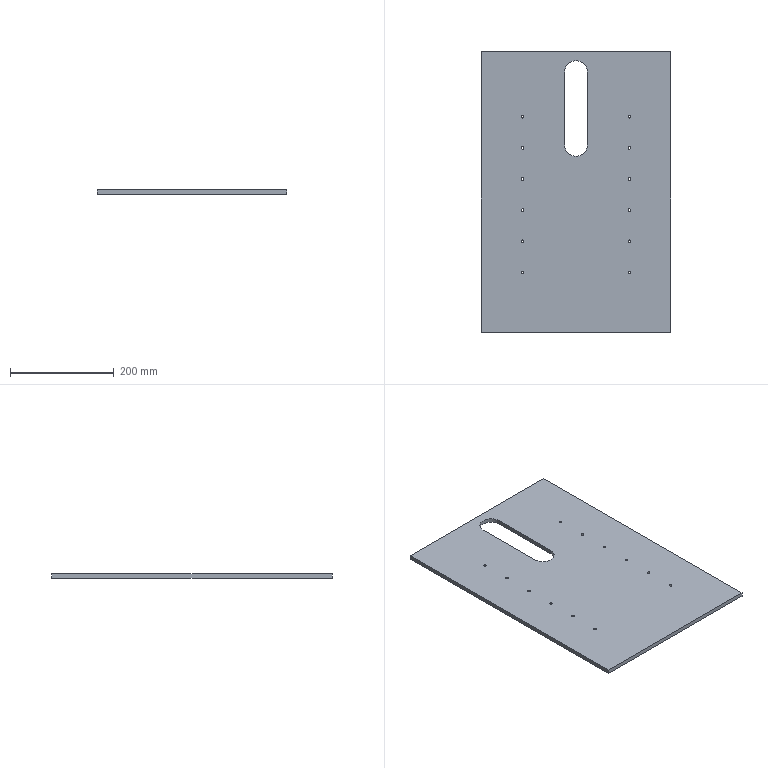Part | SolidWorks | features Extrusion 1, HoleWzd 1, LPattern 1 | 1 solid | 34 faces | box 365 x 540 x 8 mm | volume 1513471 mm3 | cylinder 26 | plane 8 | commonest cylinder face diameters 5 x24 44 x2
STEP:
#1=CARTESIAN_POINT('',(283.,-185.,0.));
#2=VERTEX_POINT('',#1);
#3=CARTESIAN_POINT('',(288.,-185.,0.));
#4=VERTEX_POINT('',#3);
#5=CARTESIAN_POINT('',(285.5,-185.,0.));
#6=DIRECTION('',(0.,0.,1.));
#7=DIRECTION('',(1.,0.,0.));
#8=AXIS2_PLACEMENT_3D('',#5,#6,#7);
#9=CIRCLE('',#8,2.5);
#10=EDGE_CURVE('',#2,#4,#9,.T.);
#11=ORIENTED_EDGE('',*,*,#10,.F.);
#12=CARTESIAN_POINT('',(283.,-185.,8.));
#13=VERTEX_POINT('',#12);
#14=CARTESIAN_POINT('',(283.,-185.,8.));
#15=DIRECTION('',(0.,0.,1.));
#16=VECTOR('',#15,1000.);
#17=LINE('',#14,#16);
#18=EDGE_CURVE('',#2,#13,#17,.T.);
#19=ORIENTED_EDGE('',*,*,#18,.T.);
#20=CARTESIAN_POINT('',(288.,-185.,8.));
#21=VERTEX_POINT('',#20);
#22=CARTESIAN_POINT('',(285.5,-185.,8.));
#23=DIRECTION('',(0.,0.,1.));
#24=DIRECTION('',(1.,0.,0.));
#25=AXIS2_PLACEMENT_3D('',#22,#23,#24);
#26=CIRCLE('',#25,2.5);
#27=EDGE_CURVE('',#13,#21,#26,.T.);
#28=ORIENTED_EDGE('',*,*,#27,.T.);
#29=CARTESIAN_POINT('',(288.,-185.,8.));
#30=DIRECTION('',(0.,0.,1.));
#31=VECTOR('',#30,1000.);
#32=LINE('',#29,#31);
#33=EDGE_CURVE('',#4,#21,#32,.T.);
#34=ORIENTED_EDGE('',*,*,#33,.F.);
#35=EDGE_LOOP('',(#11,#19,#28,#34));
#36=FACE_OUTER_BOUND('',#35,.T.);
#37=CARTESIAN_POINT('',(285.5,-185.,8.));
#38=DIRECTION('',(0.,0.,1.));
#39=DIRECTION('',(1.,0.,0.));
#40=AXIS2_PLACEMENT_3D('',#37,#38,#39);
#41=CYLINDRICAL_SURFACE('',#40,2.5);
#42=ADVANCED_FACE('',(#36),#41,.F.);
#43=CARTESIAN_POINT('',(77.,-185.,0.));
#44=VERTEX_POINT('',#43);
#45=CARTESIAN_POINT('',(82.,-185.,0.));
#46=VERTEX_POINT('',#45);
#47=CARTESIAN_POINT('',(79.5,-185.,0.));
#48=DIRECTION('',(0.,0.,1.));
#49=DIRECTION('',(1.,0.,0.));
#50=AXIS2_PLACEMENT_3D('',#47,#48,#49);
#51=CIRCLE('',#50,2.5);
#52=EDGE_CURVE('',#44,#46,#51,.T.);
#53=ORIENTED_EDGE('',*,*,#52,.F.);
#54=CARTESIAN_POINT('',(77.,-185.,8.));
#55=VERTEX_POINT('',#54);
#56=CARTESIAN_POINT('',(77.,-185.,8.));
#57=DIRECTION('',(0.,0.,1.));
#58=VECTOR('',#57,1000.);
#59=LINE('',#56,#58);
#60=EDGE_CURVE('',#44,#55,#59,.T.);
#61=ORIENTED_EDGE('',*,*,#60,.T.);
#62=CARTESIAN_POINT('',(82.,-185.,8.));
#63=VERTEX_POINT('',#62);
#64=CARTESIAN_POINT('',(79.5,-185.,8.));
#65=DIRECTION('',(0.,0.,1.));
#66=DIRECTION('',(1.,0.,0.));
#67=AXIS2_PLACEMENT_3D('',#64,#65,#66);
#68=CIRCLE('',#67,2.5);
#69=EDGE_CURVE('',#55,#63,#68,.T.);
#70=ORIENTED_EDGE('',*,*,#69,.T.);
#71=CARTESIAN_POINT('',(82.,-185.,8.));
#72=DIRECTION('',(0.,0.,1.));
#73=VECTOR('',#72,1000.);
#74=LINE('',#71,#73);
#75=EDGE_CURVE('',#46,#63,#74,.T.);
#76=ORIENTED_EDGE('',*,*,#75,.F.);
#77=EDGE_LOOP('',(#53,#61,#70,#76));
#78=FACE_OUTER_BOUND('',#77,.T.);
#79=CARTESIAN_POINT('',(79.5,-185.,8.));
#80=DIRECTION('',(0.,0.,1.));
#81=DIRECTION('',(1.,0.,0.));
#82=AXIS2_PLACEMENT_3D('',#79,#80,#81);
#83=CYLINDRICAL_SURFACE('',#82,2.5);
#84=ADVANCED_FACE('',(#78),#83,.F.);
#85=CARTESIAN_POINT('',(77.,-125.,0.));
#86=VERTEX_POINT('',#85);
#87=CARTESIAN_POINT('',(82.,-125.,0.));
#88=VERTEX_POINT('',#87);
#89=CARTESIAN_POINT('',(79.5,-125.,0.));
#90=DIRECTION('',(0.,0.,1.));
#91=DIRECTION('',(1.,0.,0.));
#92=AXIS2_PLACEMENT_3D('',#89,#90,#91);
#93=CIRCLE('',#92,2.5);
#94=EDGE_CURVE('',#86,#88,#93,.T.);
#95=ORIENTED_EDGE('',*,*,#94,.F.);
#96=CARTESIAN_POINT('',(77.,-125.,8.));
#97=VERTEX_POINT('',#96);
#98=CARTESIAN_POINT('',(77.,-125.,8.));
#99=DIRECTION('',(0.,0.,1.));
#100=VECTOR('',#99,1000.);
#101=LINE('',#98,#100);
#102=EDGE_CURVE('',#86,#97,#101,.T.);
#103=ORIENTED_EDGE('',*,*,#102,.T.);
#104=CARTESIAN_POINT('',(82.,-125.,8.));
#105=VERTEX_POINT('',#104);
#106=CARTESIAN_POINT('',(79.5,-125.,8.));
#107=DIRECTION('',(0.,0.,1.));
#108=DIRECTION('',(1.,0.,0.));
#109=AXIS2_PLACEMENT_3D('',#106,#107,#108);
#110=CIRCLE('',#109,2.5);
#111=EDGE_CURVE('',#97,#105,#110,.T.);
#112=ORIENTED_EDGE('',*,*,#111,.T.);
#113=CARTESIAN_POINT('',(82.,-125.,8.));
#114=DIRECTION('',(0.,0.,1.));
#115=VECTOR('',#114,1000.);
#116=LINE('',#113,#115);
#117=EDGE_CURVE('',#88,#105,#116,.T.);
#118=ORIENTED_EDGE('',*,*,#117,.F.);
#119=EDGE_LOOP('',(#95,#103,#112,#118));
#120=FACE_OUTER_BOUND('',#119,.T.);
#121=CARTESIAN_POINT('',(79.5,-125.,8.));
#122=DIRECTION('',(0.,0.,1.));
#123=DIRECTION('',(1.,0.,0.));
#124=AXIS2_PLACEMENT_3D('',#121,#122,#123);
#125=CYLINDRICAL_SURFACE('',#124,2.5);
#126=ADVANCED_FACE('',(#120),#125,.F.);
#127=CARTESIAN_POINT('',(283.,-125.,0.));
#128=VERTEX_POINT('',#127);
#129=CARTESIAN_POINT('',(288.,-125.,0.));
#130=VERTEX_POINT('',#129);
#131=CARTESIAN_POINT('',(285.5,-125.,0.));
#132=DIRECTION('',(0.,0.,1.));
#133=DIRECTION('',(1.,0.,0.));
#134=AXIS2_PLACEMENT_3D('',#131,#132,#133);
#135=CIRCLE('',#134,2.5);
#136=EDGE_CURVE('',#128,#130,#135,.T.);
#137=ORIENTED_EDGE('',*,*,#136,.F.);
#138=CARTESIAN_POINT('',(283.,-125.,8.));
#139=VERTEX_POINT('',#138);
#140=CARTESIAN_POINT('',(283.,-125.,8.));
#141=DIRECTION('',(0.,0.,1.));
#142=VECTOR('',#141,1000.);
#143=LINE('',#140,#142);
#144=EDGE_CURVE('',#128,#139,#143,.T.);
#145=ORIENTED_EDGE('',*,*,#144,.T.);
#146=CARTESIAN_POINT('',(288.,-125.,8.));
#147=VERTEX_POINT('',#146);
#148=CARTESIAN_POINT('',(285.5,-125.,8.));
#149=DIRECTION('',(0.,0.,1.));
#150=DIRECTION('',(1.,0.,0.));
#151=AXIS2_PLACEMENT_3D('',#148,#149,#150);
#152=CIRCLE('',#151,2.5);
#153=EDGE_CURVE('',#139,#147,#152,.T.);
#154=ORIENTED_EDGE('',*,*,#153,.T.);
#155=CARTESIAN_POINT('',(288.,-125.,8.));
#156=DIRECTION('',(0.,0.,1.));
#157=VECTOR('',#156,1000.);
#158=LINE('',#155,#157);
#159=EDGE_CURVE('',#130,#147,#158,.T.);
#160=ORIENTED_EDGE('',*,*,#159,.F.);
#161=EDGE_LOOP('',(#137,#145,#154,#160));
#162=FACE_OUTER_BOUND('',#161,.T.);
#163=CARTESIAN_POINT('',(285.5,-125.,8.));
#164=DIRECTION('',(0.,0.,1.));
#165=DIRECTION('',(1.,0.,0.));
#166=AXIS2_PLACEMENT_3D('',#163,#164,#165);
#167=CYLINDRICAL_SURFACE('',#166,2.5);
#168=ADVANCED_FACE('',(#162),#167,.F.);
#169=CARTESIAN_POINT('',(77.,-245.,0.));
#170=VERTEX_POINT('',#169);
#171=CARTESIAN_POINT('',(82.,-245.,0.));
#172=VERTEX_POINT('',#171);
#173=CARTESIAN_POINT('',(79.5,-245.,0.));
#174=DIRECTION('',(0.,0.,1.));
#175=DIRECTION('',(1.,0.,0.));
#176=AXIS2_PLACEMENT_3D('',#173,#174,#175);
#177=CIRCLE('',#176,2.5);
#178=EDGE_CURVE('',#170,#172,#177,.T.);
#179=ORIENTED_EDGE('',*,*,#178,.F.);
#180=CARTESIAN_POINT('',(77.,-245.,8.));
#181=VERTEX_POINT('',#180);
#182=CARTESIAN_POINT('',(77.,-245.,8.));
#183=DIRECTION('',(0.,0.,1.));
#184=VECTOR('',#183,1000.);
#185=LINE('',#182,#184);
#186=EDGE_CURVE('',#170,#181,#185,.T.);
#187=ORIENTED_EDGE('',*,*,#186,.T.);
#188=CARTESIAN_POINT('',(82.,-245.,8.));
#189=VERTEX_POINT('',#188);
#190=CARTESIAN_POINT('',(79.5,-245.,8.));
#191=DIRECTION('',(0.,0.,1.));
#192=DIRECTION('',(1.,0.,0.));
#193=AXIS2_PLACEMENT_3D('',#190,#191,#192);
#194=CIRCLE('',#193,2.5);
#195=EDGE_CURVE('',#181,#189,#194,.T.);
#196=ORIENTED_EDGE('',*,*,#195,.T.);
#197=CARTESIAN_POINT('',(82.,-245.,8.));
#198=DIRECTION('',(0.,0.,1.));
#199=VECTOR('',#198,1000.);
#200=LINE('',#197,#199);
#201=EDGE_CURVE('',#172,#189,#200,.T.);
#202=ORIENTED_EDGE('',*,*,#201,.F.);
#203=EDGE_LOOP('',(#179,#187,#196,#202));
#204=FACE_OUTER_BOUND('',#203,.T.);
#205=CARTESIAN_POINT('',(79.5,-245.,8.));
#206=DIRECTION('',(0.,0.,1.));
#207=DIRECTION('',(1.,0.,0.));
#208=AXIS2_PLACEMENT_3D('',#205,#206,#207);
#209=CYLINDRICAL_SURFACE('',#208,2.5);
#210=ADVANCED_FACE('',(#204),#209,.F.);
#211=CARTESIAN_POINT('',(77.,-305.,0.));
#212=VERTEX_POINT('',#211);
#213=CARTESIAN_POINT('',(82.,-305.,0.));
#214=VERTEX_POINT('',#213);
#215=CARTESIAN_POINT('',(79.5,-305.,0.));
#216=DIRECTION('',(0.,0.,1.));
#217=DIRECTION('',(1.,0.,0.));
#218=AXIS2_PLACEMENT_3D('',#215,#216,#217);
#219=CIRCLE('',#218,2.5);
#220=EDGE_CURVE('',#212,#214,#219,.T.);
#221=ORIENTED_EDGE('',*,*,#220,.F.);
#222=CARTESIAN_POINT('',(77.,-305.,8.));
#223=VERTEX_POINT('',#222);
#224=CARTESIAN_POINT('',(77.,-305.,8.));
#225=DIRECTION('',(0.,0.,1.));
#226=VECTOR('',#225,1000.);
#227=LINE('',#224,#226);
#228=EDGE_CURVE('',#212,#223,#227,.T.);
#229=ORIENTED_EDGE('',*,*,#228,.T.);
#230=CARTESIAN_POINT('',(82.,-305.,8.));
#231=VERTEX_POINT('',#230);
#232=CARTESIAN_POINT('',(79.5,-305.,8.));
#233=DIRECTION('',(0.,0.,1.));
#234=DIRECTION('',(1.,0.,0.));
#235=AXIS2_PLACEMENT_3D('',#232,#233,#234);
#236=CIRCLE('',#235,2.5);
#237=EDGE_CURVE('',#223,#231,#236,.T.);
#238=ORIENTED_EDGE('',*,*,#237,.T.);
#239=CARTESIAN_POINT('',(82.,-305.,8.));
#240=DIRECTION('',(0.,0.,1.));
#241=VECTOR('',#240,1000.);
#242=LINE('',#239,#241);
#243=EDGE_CURVE('',#214,#231,#242,.T.);
#244=ORIENTED_EDGE('',*,*,#243,.F.);
#245=EDGE_LOOP('',(#221,#229,#238,#244));
#246=FACE_OUTER_BOUND('',#245,.T.);
#247=CARTESIAN_POINT('',(79.5,-305.,8.));
#248=DIRECTION('',(0.,0.,1.));
#249=DIRECTION('',(1.,0.,0.));
#250=AXIS2_PLACEMENT_3D('',#247,#248,#249);
#251=CYLINDRICAL_SURFACE('',#250,2.5);
#252=ADVANCED_FACE('',(#246),#251,.F.);
#253=CARTESIAN_POINT('',(77.,-365.,0.));
#254=VERTEX_POINT('',#253);
#255=CARTESIAN_POINT('',(82.,-365.,0.));
#256=VERTEX_POINT('',#255);
#257=CARTESIAN_POINT('',(79.5,-365.,0.));
#258=DIRECTION('',(0.,0.,1.));
#259=DIRECTION('',(1.,0.,0.));
#260=AXIS2_PLACEMENT_3D('',#257,#258,#259);
#261=CIRCLE('',#260,2.5);
#262=EDGE_CURVE('',#254,#256,#261,.T.);
#263=ORIENTED_EDGE('',*,*,#262,.F.);
#264=CARTESIAN_POINT('',(77.,-365.,8.));
#265=VERTEX_POINT('',#264);
#266=CARTESIAN_POINT('',(77.,-365.,8.));
#267=DIRECTION('',(0.,0.,1.));
#268=VECTOR('',#267,1000.);
#269=LINE('',#266,#268);
#270=EDGE_CURVE('',#254,#265,#269,.T.);
#271=ORIENTED_EDGE('',*,*,#270,.T.);
#272=CARTESIAN_POINT('',(82.,-365.,8.));
#273=VERTEX_POINT('',#272);
#274=CARTESIAN_POINT('',(79.5,-365.,8.));
#275=DIRECTION('',(0.,0.,1.));
#276=DIRECTION('',(1.,0.,0.));
#277=AXIS2_PLACEMENT_3D('',#274,#275,#276);
#278=CIRCLE('',#277,2.5);
#279=EDGE_CURVE('',#265,#273,#278,.T.);
#280=ORIENTED_EDGE('',*,*,#279,.T.);
#281=CARTESIAN_POINT('',(82.,-365.,8.));
#282=DIRECTION('',(0.,0.,1.));
#283=VECTOR('',#282,1000.);
#284=LINE('',#281,#283);
#285=EDGE_CURVE('',#256,#273,#284,.T.);
#286=ORIENTED_EDGE('',*,*,#285,.F.);
#287=EDGE_LOOP('',(#263,#271,#280,#286));
#288=FACE_OUTER_BOUND('',#287,.T.);
#289=CARTESIAN_POINT('',(79.5,-365.,8.));
#290=DIRECTION('',(0.,0.,1.));
#291=DIRECTION('',(1.,0.,0.));
#292=AXIS2_PLACEMENT_3D('',#289,#290,#291);
#293=CYLINDRICAL_SURFACE('',#292,2.5);
#294=ADVANCED_FACE('',(#288),#293,.F.);
#295=CARTESIAN_POINT('',(77.,-425.,0.));
#296=VERTEX_POINT('',#295);
#297=CARTESIAN_POINT('',(82.,-425.,0.));
#298=VERTEX_POINT('',#297);
#299=CARTESIAN_POINT('',(79.5,-425.,0.));
#300=DIRECTION('',(0.,0.,1.));
#301=DIRECTION('',(1.,0.,0.));
#302=AXIS2_PLACEMENT_3D('',#299,#300,#301);
#303=CIRCLE('',#302,2.5);
#304=EDGE_CURVE('',#296,#298,#303,.T.);
#305=ORIENTED_EDGE('',*,*,#304,.F.);
#306=CARTESIAN_POINT('',(77.,-425.,8.));
#307=VERTEX_POINT('',#306);
#308=CARTESIAN_POINT('',(77.,-425.,8.));
#309=DIRECTION('',(0.,0.,1.));
#310=VECTOR('',#309,1000.);
#311=LINE('',#308,#310);
#312=EDGE_CURVE('',#296,#307,#311,.T.);
#313=ORIENTED_EDGE('',*,*,#312,.T.);
#314=CARTESIAN_POINT('',(82.,-425.,8.));
#315=VERTEX_POINT('',#314);
#316=CARTESIAN_POINT('',(79.5,-425.,8.));
#317=DIRECTION('',(0.,0.,1.));
#318=DIRECTION('',(1.,0.,0.));
#319=AXIS2_PLACEMENT_3D('',#316,#317,#318);
#320=CIRCLE('',#319,2.5);
#321=EDGE_CURVE('',#307,#315,#320,.T.);
#322=ORIENTED_EDGE('',*,*,#321,.T.);
#323=CARTESIAN_POINT('',(82.,-425.,8.));
#324=DIRECTION('',(0.,0.,1.));
#325=VECTOR('',#324,1000.);
#326=LINE('',#323,#325);
#327=EDGE_CURVE('',#298,#315,#326,.T.);
#328=ORIENTED_EDGE('',*,*,#327,.F.);
#329=EDGE_LOOP('',(#305,#313,#322,#328));
#330=FACE_OUTER_BOUND('',#329,.T.);
#331=CARTESIAN_POINT('',(79.5,-425.,8.));
#332=DIRECTION('',(0.,0.,1.));
#333=DIRECTION('',(1.,0.,0.));
#334=AXIS2_PLACEMENT_3D('',#331,#332,#333);
#335=CYLINDRICAL_SURFACE('',#334,2.5);
#336=ADVANCED_FACE('',(#330),#335,.F.);
#337=CARTESIAN_POINT('',(283.,-245.,0.));
#338=VERTEX_POINT('',#337);
#339=CARTESIAN_POINT('',(288.,-245.,0.));
#340=VERTEX_POINT('',#339);
#341=CARTESIAN_POINT('',(285.5,-245.,0.));
#342=DIRECTION('',(0.,0.,1.));
#343=DIRECTION('',(1.,0.,0.));
#344=AXIS2_PLACEMENT_3D('',#341,#342,#343);
#345=CIRCLE('',#344,2.5);
#346=EDGE_CURVE('',#338,#340,#345,.T.);
#347=ORIENTED_EDGE('',*,*,#346,.F.);
#348=CARTESIAN_POINT('',(283.,-245.,8.));
#349=VERTEX_POINT('',#348);
#350=CARTESIAN_POINT('',(283.,-245.,8.));
#351=DIRECTION('',(0.,0.,1.));
#352=VECTOR('',#351,1000.);
#353=LINE('',#350,#352);
#354=EDGE_CURVE('',#338,#349,#353,.T.);
#355=ORIENTED_EDGE('',*,*,#354,.T.);
#356=CARTESIAN_POINT('',(288.,-245.,8.));
#357=VERTEX_POINT('',#356);
#358=CARTESIAN_POINT('',(285.5,-245.,8.));
#359=DIRECTION('',(0.,0.,1.));
#360=DIRECTION('',(1.,0.,0.));
#361=AXIS2_PLACEMENT_3D('',#358,#359,#360);
#362=CIRCLE('',#361,2.5);
#363=EDGE_CURVE('',#349,#357,#362,.T.);
#364=ORIENTED_EDGE('',*,*,#363,.T.);
#365=CARTESIAN_POINT('',(288.,-245.,8.));
#366=DIRECTION('',(0.,0.,1.));
#367=VECTOR('',#366,1000.);
#368=LINE('',#365,#367);
#369=EDGE_CURVE('',#340,#357,#368,.T.);
#370=ORIENTED_EDGE('',*,*,#369,.F.);
#371=EDGE_LOOP('',(#347,#355,#364,#370));
#372=FACE_OUTER_BOUND('',#371,.T.);
#373=CARTESIAN_POINT('',(285.5,-245.,8.));
#374=DIRECTION('',(0.,0.,1.));
#375=DIRECTION('',(1.,0.,0.));
#376=AXIS2_PLACEMENT_3D('',#373,#374,#375);
#377=CYLINDRICAL_SURFACE('',#376,2.5);
#378=ADVANCED_FACE('',(#372),#377,.F.);
#379=CARTESIAN_POINT('',(283.,-305.,0.));
#380=VERTEX_POINT('',#379);
#381=CARTESIAN_POINT('',(288.,-305.,0.));
#382=VERTEX_POINT('',#381);
#383=CARTESIAN_POINT('',(285.5,-305.,0.));
#384=DIRECTION('',(0.,0.,1.));
#385=DIRECTION('',(1.,0.,0.));
#386=AXIS2_PLACEMENT_3D('',#383,#384,#385);
#387=CIRCLE('',#386,2.5);
#388=EDGE_CURVE('',#380,#382,#387,.T.);
#389=ORIENTED_EDGE('',*,*,#388,.F.);
#390=CARTESIAN_POINT('',(283.,-305.,8.));
#391=VERTEX_POINT('',#390);
#392=CARTESIAN_POINT('',(283.,-305.,8.));
#393=DIRECTION('',(0.,0.,1.));
#394=VECTOR('',#393,1000.);
#395=LINE('',#392,#394);
#396=EDGE_CURVE('',#380,#391,#395,.T.);
#397=ORIENTED_EDGE('',*,*,#396,.T.);
#398=CARTESIAN_POINT('',(288.,-305.,8.));
#399=VERTEX_POINT('',#398);
#400=CARTESIAN_POINT('',(285.5,-305.,8.));
#401=DIRECTION('',(0.,0.,1.));
#402=DIRECTION('',(1.,0.,0.));
#403=AXIS2_PLACEMENT_3D('',#400,#401,#402);
#404=CIRCLE('',#403,2.5);
#405=EDGE_CURVE('',#391,#399,#404,.T.);
#406=ORIENTED_EDGE('',*,*,#405,.T.);
#407=CARTESIAN_POINT('',(288.,-305.,8.));
#408=DIRECTION('',(0.,0.,1.));
#409=VECTOR('',#408,1000.);
#410=LINE('',#407,#409);
#411=EDGE_CURVE('',#382,#399,#410,.T.);
#412=ORIENTED_EDGE('',*,*,#411,.F.);
#413=EDGE_LOOP('',(#389,#397,#406,#412));
#414=FACE_OUTER_BOUND('',#413,.T.);
#415=CARTESIAN_POINT('',(285.5,-305.,8.));
#416=DIRECTION('',(0.,0.,1.));
#417=DIRECTION('',(1.,0.,0.));
#418=AXIS2_PLACEMENT_3D('',#415,#416,#417);
#419=CYLINDRICAL_SURFACE('',#418,2.5);
#420=ADVANCED_FACE('',(#414),#419,.F.);
#421=CARTESIAN_POINT('',(283.,-365.,0.));
#422=VERTEX_POINT('',#421);
#423=CARTESIAN_POINT('',(288.,-365.,0.));
#424=VERTEX_POINT('',#423);
#425=CARTESIAN_POINT('',(285.5,-365.,0.));
#426=DIRECTION('',(0.,0.,1.));
#427=DIRECTION('',(1.,0.,0.));
#428=AXIS2_PLACEMENT_3D('',#425,#426,#427);
#429=CIRCLE('',#428,2.5);
#430=EDGE_CURVE('',#422,#424,#429,.T.);
#431=ORIENTED_EDGE('',*,*,#430,.F.);
#432=CARTESIAN_POINT('',(283.,-365.,8.));
#433=VERTEX_POINT('',#432);
#434=CARTESIAN_POINT('',(283.,-365.,8.));
#435=DIRECTION('',(0.,0.,1.));
#436=VECTOR('',#435,1000.);
#437=LINE('',#434,#436);
#438=EDGE_CURVE('',#422,#433,#437,.T.);
#439=ORIENTED_EDGE('',*,*,#438,.T.);
#440=CARTESIAN_POINT('',(288.,-365.,8.));
#441=VERTEX_POINT('',#440);
#442=CARTESIAN_POINT('',(285.5,-365.,8.));
#443=DIRECTION('',(0.,0.,1.));
#444=DIRECTION('',(1.,0.,0.));
#445=AXIS2_PLACEMENT_3D('',#442,#443,#444);
#446=CIRCLE('',#445,2.5);
#447=EDGE_CURVE('',#433,#441,#446,.T.);
#448=ORIENTED_EDGE('',*,*,#447,.T.);
#449=CARTESIAN_POINT('',(288.,-365.,8.));
#450=DIRECTION('',(0.,0.,1.));
#451=VECTOR('',#450,1000.);
#452=LINE('',#449,#451);
#453=EDGE_CURVE('',#424,#441,#452,.T.);
#454=ORIENTED_EDGE('',*,*,#453,.F.);
#455=EDGE_LOOP('',(#431,#439,#448,#454));
#456=FACE_OUTER_BOUND('',#455,.T.);
#457=CARTESIAN_POINT('',(285.5,-365.,8.));
#458=DIRECTION('',(0.,0.,1.));
#459=DIRECTION('',(1.,0.,0.));
#460=AXIS2_PLACEMENT_3D('',#457,#458,#459);
#461=CYLINDRICAL_SURFACE('',#460,2.5);
#462=ADVANCED_FACE('',(#456),#461,.F.);
#463=CARTESIAN_POINT('',(283.,-425.,0.));
#464=VERTEX_POINT('',#463);
#465=CARTESIAN_POINT('',(288.,-425.,0.));
#466=VERTEX_POINT('',#465);
#467=CARTESIAN_POINT('',(285.5,-425.,0.));
#468=DIRECTION('',(0.,0.,1.));
#469=DIRECTION('',(1.,0.,0.));
#470=AXIS2_PLACEMENT_3D('',#467,#468,#469);
#471=CIRCLE('',#470,2.5);
#472=EDGE_CURVE('',#464,#466,#471,.T.);
#473=ORIENTED_EDGE('',*,*,#472,.F.);
#474=CARTESIAN_POINT('',(283.,-425.,8.));
#475=VERTEX_POINT('',#474);
#476=CARTESIAN_POINT('',(283.,-425.,8.));
#477=DIRECTION('',(0.,0.,1.));
#478=VECTOR('',#477,1000.);
#479=LINE('',#476,#478);
#480=EDGE_CURVE('',#464,#475,#479,.T.);
#481=ORIENTED_EDGE('',*,*,#480,.T.);
#482=CARTESIAN_POINT('',(288.,-425.,8.));
#483=VERTEX_POINT('',#482);
#484=CARTESIAN_POINT('',(285.5,-425.,8.));
#485=DIRECTION('',(0.,0.,1.));
#486=DIRECTION('',(1.,0.,0.));
#487=AXIS2_PLACEMENT_3D('',#484,#485,#486);
#488=CIRCLE('',#487,2.5);
#489=EDGE_CURVE('',#475,#483,#488,.T.);
#490=ORIENTED_EDGE('',*,*,#489,.T.);
#491=CARTESIAN_POINT('',(288.,-425.,8.));
#492=DIRECTION('',(0.,0.,1.));
#493=VECTOR('',#492,1000.);
#494=LINE('',#491,#493);
#495=EDGE_CURVE('',#466,#483,#494,.T.);
#496=ORIENTED_EDGE('',*,*,#495,.F.);
#497=EDGE_LOOP('',(#473,#481,#490,#496));
#498=FACE_OUTER_BOUND('',#497,.T.);
#499=CARTESIAN_POINT('',(285.5,-425.,8.));
#500=DIRECTION('',(0.,0.,1.));
#501=DIRECTION('',(1.,0.,0.));
#502=AXIS2_PLACEMENT_3D('',#499,#500,#501);
#503=CYLINDRICAL_SURFACE('',#502,2.5);
#504=ADVANCED_FACE('',(#498),#503,.F.);
#505=ORIENTED_EDGE('',*,*,#480,.F.);
#506=CARTESIAN_POINT('',(285.5,-425.,0.));
#507=DIRECTION('',(0.,0.,1.));
#508=DIRECTION('',(1.,0.,0.));
#509=AXIS2_PLACEMENT_3D('',#506,#507,#508);
#510=CIRCLE('',#509,2.5);
#511=EDGE_CURVE('',#466,#464,#510,.T.);
#512=ORIENTED_EDGE('',*,*,#511,.F.);
#513=ORIENTED_EDGE('',*,*,#495,.T.);
#514=CARTESIAN_POINT('',(285.5,-425.,8.));
#515=DIRECTION('',(0.,0.,1.));
#516=DIRECTION('',(1.,0.,0.));
#517=AXIS2_PLACEMENT_3D('',#514,#515,#516);
#518=CIRCLE('',#517,2.5);
#519=EDGE_CURVE('',#483,#475,#518,.T.);
#520=ORIENTED_EDGE('',*,*,#519,.T.);
#521=EDGE_LOOP('',(#505,#512,#513,#520));
#522=FACE_OUTER_BOUND('',#521,.T.);
#523=CARTESIAN_POINT('',(285.5,-425.,8.));
#524=DIRECTION('',(0.,0.,1.));
#525=DIRECTION('',(1.,0.,0.));
#526=AXIS2_PLACEMENT_3D('',#523,#524,#525);
#527=CYLINDRICAL_SURFACE('',#526,2.5);
#528=ADVANCED_FACE('',(#522),#527,.F.);
#529=ORIENTED_EDGE('',*,*,#438,.F.);
#530=CARTESIAN_POINT('',(285.5,-365.,0.));
#531=DIRECTION('',(0.,0.,1.));
#532=DIRECTION('',(1.,0.,0.));
#533=AXIS2_PLACEMENT_3D('',#530,#531,#532);
#534=CIRCLE('',#533,2.5);
#535=EDGE_CURVE('',#424,#422,#534,.T.);
#536=ORIENTED_EDGE('',*,*,#535,.F.);
#537=ORIENTED_EDGE('',*,*,#453,.T.);
#538=CARTESIAN_POINT('',(285.5,-365.,8.));
#539=DIRECTION('',(0.,0.,1.));
#540=DIRECTION('',(1.,0.,0.));
#541=AXIS2_PLACEMENT_3D('',#538,#539,#540);
#542=CIRCLE('',#541,2.5);
#543=EDGE_CURVE('',#441,#433,#542,.T.);
#544=ORIENTED_EDGE('',*,*,#543,.T.);
#545=EDGE_LOOP('',(#529,#536,#537,#544));
#546=FACE_OUTER_BOUND('',#545,.T.);
#547=CARTESIAN_POINT('',(285.5,-365.,8.));
#548=DIRECTION('',(0.,0.,1.));
#549=DIRECTION('',(1.,0.,0.));
#550=AXIS2_PLACEMENT_3D('',#547,#548,#549);
#551=CYLINDRICAL_SURFACE('',#550,2.5);
#552=ADVANCED_FACE('',(#546),#551,.F.);
#553=ORIENTED_EDGE('',*,*,#396,.F.);
#554=CARTESIAN_POINT('',(285.5,-305.,0.));
#555=DIRECTION('',(0.,0.,1.));
#556=DIRECTION('',(1.,0.,0.));
#557=AXIS2_PLACEMENT_3D('',#554,#555,#556);
#558=CIRCLE('',#557,2.5);
#559=EDGE_CURVE('',#382,#380,#558,.T.);
#560=ORIENTED_EDGE('',*,*,#559,.F.);
#561=ORIENTED_EDGE('',*,*,#411,.T.);
#562=CARTESIAN_POINT('',(285.5,-305.,8.));
#563=DIRECTION('',(0.,0.,1.));
#564=DIRECTION('',(1.,0.,0.));
#565=AXIS2_PLACEMENT_3D('',#562,#563,#564);
#566=CIRCLE('',#565,2.5);
#567=EDGE_CURVE('',#399,#391,#566,.T.);
#568=ORIENTED_EDGE('',*,*,#567,.T.);
#569=EDGE_LOOP('',(#553,#560,#561,#568));
#570=FACE_OUTER_BOUND('',#569,.T.);
#571=CARTESIAN_POINT('',(285.5,-305.,8.));
#572=DIRECTION('',(0.,0.,1.));
#573=DIRECTION('',(1.,0.,0.));
#574=AXIS2_PLACEMENT_3D('',#571,#572,#573);
#575=CYLINDRICAL_SURFACE('',#574,2.5);
#576=ADVANCED_FACE('',(#570),#575,.F.);
#577=ORIENTED_EDGE('',*,*,#354,.F.);
#578=CARTESIAN_POINT('',(285.5,-245.,0.));
#579=DIRECTION('',(0.,0.,1.));
#580=DIRECTION('',(1.,0.,0.));
#581=AXIS2_PLACEMENT_3D('',#578,#579,#580);
#582=CIRCLE('',#581,2.5);
#583=EDGE_CURVE('',#340,#338,#582,.T.);
#584=ORIENTED_EDGE('',*,*,#583,.F.);
#585=ORIENTED_EDGE('',*,*,#369,.T.);
#586=CARTESIAN_POINT('',(285.5,-245.,8.));
#587=DIRECTION('',(0.,0.,1.));
#588=DIRECTION('',(1.,0.,0.));
#589=AXIS2_PLACEMENT_3D('',#586,#587,#588);
#590=CIRCLE('',#589,2.5);
#591=EDGE_CURVE('',#357,#349,#590,.T.);
#592=ORIENTED_EDGE('',*,*,#591,.T.);
#593=EDGE_LOOP('',(#577,#584,#585,#592));
#594=FACE_OUTER_BOUND('',#593,.T.);
#595=CARTESIAN_POINT('',(285.5,-245.,8.));
#596=DIRECTION('',(0.,0.,1.));
#597=DIRECTION('',(1.,0.,0.));
#598=AXIS2_PLACEMENT_3D('',#595,#596,#597);
#599=CYLINDRICAL_SURFACE('',#598,2.5);
#600=ADVANCED_FACE('',(#594),#599,.F.);
#601=ORIENTED_EDGE('',*,*,#312,.F.);
#602=CARTESIAN_POINT('',(79.5,-425.,0.));
#603=DIRECTION('',(0.,0.,1.));
#604=DIRECTION('',(1.,0.,0.));
#605=AXIS2_PLACEMENT_3D('',#602,#603,#604);
#606=CIRCLE('',#605,2.5);
#607=EDGE_CURVE('',#298,#296,#606,.T.);
#608=ORIENTED_EDGE('',*,*,#607,.F.);
#609=ORIENTED_EDGE('',*,*,#327,.T.);
#610=CARTESIAN_POINT('',(79.5,-425.,8.));
#611=DIRECTION('',(0.,0.,1.));
#612=DIRECTION('',(1.,0.,0.));
#613=AXIS2_PLACEMENT_3D('',#610,#611,#612);
#614=CIRCLE('',#613,2.5);
#615=EDGE_CURVE('',#315,#307,#614,.T.);
#616=ORIENTED_EDGE('',*,*,#615,.T.);
#617=EDGE_LOOP('',(#601,#608,#609,#616));
#618=FACE_OUTER_BOUND('',#617,.T.);
#619=CARTESIAN_POINT('',(79.5,-425.,8.));
#620=DIRECTION('',(0.,0.,1.));
#621=DIRECTION('',(1.,0.,0.));
#622=AXIS2_PLACEMENT_3D('',#619,#620,#621);
#623=CYLINDRICAL_SURFACE('',#622,2.5);
#624=ADVANCED_FACE('',(#618),#623,.F.);
#625=ORIENTED_EDGE('',*,*,#270,.F.);
#626=CARTESIAN_POINT('',(79.5,-365.,0.));
#627=DIRECTION('',(0.,0.,1.));
#628=DIRECTION('',(1.,0.,0.));
#629=AXIS2_PLACEMENT_3D('',#626,#627,#628);
#630=CIRCLE('',#629,2.5);
#631=EDGE_CURVE('',#256,#254,#630,.T.);
#632=ORIENTED_EDGE('',*,*,#631,.F.);
#633=ORIENTED_EDGE('',*,*,#285,.T.);
#634=CARTESIAN_POINT('',(79.5,-365.,8.));
#635=DIRECTION('',(0.,0.,1.));
#636=DIRECTION('',(1.,0.,0.));
#637=AXIS2_PLACEMENT_3D('',#634,#635,#636);
#638=CIRCLE('',#637,2.5);
#639=EDGE_CURVE('',#273,#265,#638,.T.);
#640=ORIENTED_EDGE('',*,*,#639,.T.);
#641=EDGE_LOOP('',(#625,#632,#633,#640));
#642=FACE_OUTER_BOUND('',#641,.T.);
#643=CARTESIAN_POINT('',(79.5,-365.,8.));
#644=DIRECTION('',(0.,0.,1.));
#645=DIRECTION('',(1.,0.,0.));
#646=AXIS2_PLACEMENT_3D('',#643,#644,#645);
#647=CYLINDRICAL_SURFACE('',#646,2.5);
#648=ADVANCED_FACE('',(#642),#647,.F.);
#649=ORIENTED_EDGE('',*,*,#228,.F.);
#650=CARTESIAN_POINT('',(79.5,-305.,0.));
#651=DIRECTION('',(0.,0.,1.));
#652=DIRECTION('',(1.,0.,0.));
#653=AXIS2_PLACEMENT_3D('',#650,#651,#652);
#654=CIRCLE('',#653,2.5);
#655=EDGE_CURVE('',#214,#212,#654,.T.);
#656=ORIENTED_EDGE('',*,*,#655,.F.);
#657=ORIENTED_EDGE('',*,*,#243,.T.);
#658=CARTESIAN_POINT('',(79.5,-305.,8.));
#659=DIRECTION('',(0.,0.,1.));
#660=DIRECTION('',(1.,0.,0.));
#661=AXIS2_PLACEMENT_3D('',#658,#659,#660);
#662=CIRCLE('',#661,2.5);
#663=EDGE_CURVE('',#231,#223,#662,.T.);
#664=ORIENTED_EDGE('',*,*,#663,.T.);
#665=EDGE_LOOP('',(#649,#656,#657,#664));
#666=FACE_OUTER_BOUND('',#665,.T.);
#667=CARTESIAN_POINT('',(79.5,-305.,8.));
#668=DIRECTION('',(0.,0.,1.));
#669=DIRECTION('',(1.,0.,0.));
#670=AXIS2_PLACEMENT_3D('',#667,#668,#669);
#671=CYLINDRICAL_SURFACE('',#670,2.5);
#672=ADVANCED_FACE('',(#666),#671,.F.);
#673=ORIENTED_EDGE('',*,*,#186,.F.);
#674=CARTESIAN_POINT('',(79.5,-245.,0.));
#675=DIRECTION('',(0.,0.,1.));
#676=DIRECTION('',(1.,0.,0.));
#677=AXIS2_PLACEMENT_3D('',#674,#675,#676);
#678=CIRCLE('',#677,2.5);
#679=EDGE_CURVE('',#172,#170,#678,.T.);
#680=ORIENTED_EDGE('',*,*,#679,.F.);
#681=ORIENTED_EDGE('',*,*,#201,.T.);
#682=CARTESIAN_POINT('',(79.5,-245.,8.));
#683=DIRECTION('',(0.,0.,1.));
#684=DIRECTION('',(1.,0.,0.));
#685=AXIS2_PLACEMENT_3D('',#682,#683,#684);
#686=CIRCLE('',#685,2.5);
#687=EDGE_CURVE('',#189,#181,#686,.T.);
#688=ORIENTED_EDGE('',*,*,#687,.T.);
#689=EDGE_LOOP('',(#673,#680,#681,#688));
#690=FACE_OUTER_BOUND('',#689,.T.);
#691=CARTESIAN_POINT('',(79.5,-245.,8.));
#692=DIRECTION('',(0.,0.,1.));
#693=DIRECTION('',(1.,0.,0.));
#694=AXIS2_PLACEMENT_3D('',#691,#692,#693);
#695=CYLINDRICAL_SURFACE('',#694,2.5);
#696=ADVANCED_FACE('',(#690),#695,.F.);
#697=CARTESIAN_POINT('',(285.5,-185.,8.));
#698=DIRECTION('',(0.,0.,1.));
#699=DIRECTION('',(1.,0.,0.));
#700=AXIS2_PLACEMENT_3D('',#697,#698,#699);
#701=CIRCLE('',#700,2.5);
#702=EDGE_CURVE('',#21,#13,#701,.T.);
#703=ORIENTED_EDGE('',*,*,#702,.F.);
#704=ORIENTED_EDGE('',*,*,#27,.F.);
#705=EDGE_LOOP('',(#703,#704));
#706=FACE_BOUND('',#705,.T.);
#707=CARTESIAN_POINT('',(79.5,-185.,8.));
#708=DIRECTION('',(0.,0.,1.));
#709=DIRECTION('',(1.,0.,0.));
#710=AXIS2_PLACEMENT_3D('',#707,#708,#709);
#711=CIRCLE('',#710,2.5);
#712=EDGE_CURVE('',#63,#55,#711,.T.);
#713=ORIENTED_EDGE('',*,*,#712,.F.);
#714=ORIENTED_EDGE('',*,*,#69,.F.);
#715=EDGE_LOOP('',(#713,#714));
#716=FACE_BOUND('',#715,.T.);
#717=CARTESIAN_POINT('',(79.5,-125.,8.));
#718=DIRECTION('',(0.,0.,1.));
#719=DIRECTION('',(1.,0.,0.));
#720=AXIS2_PLACEMENT_3D('',#717,#718,#719);
#721=CIRCLE('',#720,2.5);
#722=EDGE_CURVE('',#105,#97,#721,.T.);
#723=ORIENTED_EDGE('',*,*,#722,.F.);
#724=ORIENTED_EDGE('',*,*,#111,.F.);
#725=EDGE_LOOP('',(#723,#724));
#726=FACE_BOUND('',#725,.T.);
#727=CARTESIAN_POINT('',(285.5,-125.,8.));
#728=DIRECTION('',(0.,0.,1.));
#729=DIRECTION('',(1.,0.,0.));
#730=AXIS2_PLACEMENT_3D('',#727,#728,#729);
#731=CIRCLE('',#730,2.5);
#732=EDGE_CURVE('',#147,#139,#731,.T.);
#733=ORIENTED_EDGE('',*,*,#732,.F.);
#734=ORIENTED_EDGE('',*,*,#153,.F.);
#735=EDGE_LOOP('',(#733,#734));
#736=FACE_BOUND('',#735,.T.);
#737=CARTESIAN_POINT('',(0.,0.,8.));
#738=VERTEX_POINT('',#737);
#739=CARTESIAN_POINT('',(0.,-540.,8.));
#740=VERTEX_POINT('',#739);
#741=CARTESIAN_POINT('',(0.,0.,8.));
#742=DIRECTION('',(0.,-1.,0.));
#743=VECTOR('',#742,1000.);
#744=LINE('',#741,#743);
#745=EDGE_CURVE('',#738,#740,#744,.T.);
#746=ORIENTED_EDGE('',*,*,#745,.T.);
#747=CARTESIAN_POINT('',(365.,-540.,8.));
#748=VERTEX_POINT('',#747);
#749=CARTESIAN_POINT('',(0.,-540.,8.));
#750=DIRECTION('',(1.,0.,0.));
#751=VECTOR('',#750,1000.);
#752=LINE('',#749,#751);
#753=EDGE_CURVE('',#740,#748,#752,.T.);
#754=ORIENTED_EDGE('',*,*,#753,.T.);
#755=CARTESIAN_POINT('',(365.,0.,8.));
#756=VERTEX_POINT('',#755);
#757=CARTESIAN_POINT('',(365.,0.,8.));
#758=DIRECTION('',(0.,1.,0.));
#759=VECTOR('',#758,1000.);
#760=LINE('',#757,#759);
#761=EDGE_CURVE('',#748,#756,#760,.T.);
#762=ORIENTED_EDGE('',*,*,#761,.T.);
#763=CARTESIAN_POINT('',(0.,0.,8.));
#764=DIRECTION('',(-1.,0.,0.));
#765=VECTOR('',#764,1000.);
#766=LINE('',#763,#765);
#767=EDGE_CURVE('',#756,#738,#766,.T.);
#768=ORIENTED_EDGE('',*,*,#767,.T.);
#769=EDGE_LOOP('',(#746,#754,#762,#768));
#770=FACE_OUTER_BOUND('',#769,.T.);
#771=CARTESIAN_POINT('',(160.5,-39.,8.));
#772=VERTEX_POINT('',#771);
#773=CARTESIAN_POINT('',(160.5,-179.,8.));
#774=VERTEX_POINT('',#773);
#775=CARTESIAN_POINT('',(160.5,-39.,8.));
#776=DIRECTION('',(0.,-1.,0.));
#777=VECTOR('',#776,1000.);
#778=LINE('',#775,#777);
#779=EDGE_CURVE('',#772,#774,#778,.T.);
#780=ORIENTED_EDGE('',*,*,#779,.F.);
#781=CARTESIAN_POINT('',(204.5,-39.,8.));
#782=VERTEX_POINT('',#781);
#783=CARTESIAN_POINT('',(182.5,-39.,8.));
#784=DIRECTION('',(0.,0.,1.));
#785=DIRECTION('',(1.,0.,0.));
#786=AXIS2_PLACEMENT_3D('',#783,#784,#785);
#787=CIRCLE('',#786,22.);
#788=EDGE_CURVE('',#782,#772,#787,.T.);
#789=ORIENTED_EDGE('',*,*,#788,.F.);
#790=CARTESIAN_POINT('',(204.5,-179.,8.));
#791=VERTEX_POINT('',#790);
#792=CARTESIAN_POINT('',(204.5,-39.,8.));
#793=DIRECTION('',(0.,1.,0.));
#794=VECTOR('',#793,1000.);
#795=LINE('',#792,#794);
#796=EDGE_CURVE('',#791,#782,#795,.T.);
#797=ORIENTED_EDGE('',*,*,#796,.F.);
#798=CARTESIAN_POINT('',(182.5,-179.,8.));
#799=DIRECTION('',(0.,0.,1.));
#800=DIRECTION('',(1.,0.,0.));
#801=AXIS2_PLACEMENT_3D('',#798,#799,#800);
#802=CIRCLE('',#801,22.);
#803=EDGE_CURVE('',#774,#791,#802,.T.);
#804=ORIENTED_EDGE('',*,*,#803,.F.);
#805=EDGE_LOOP('',(#780,#789,#797,#804));
#806=FACE_BOUND('',#805,.T.);
#807=ORIENTED_EDGE('',*,*,#687,.F.);
#808=ORIENTED_EDGE('',*,*,#195,.F.);
#809=EDGE_LOOP('',(#807,#808));
#810=FACE_BOUND('',#809,.T.);
#811=ORIENTED_EDGE('',*,*,#663,.F.);
#812=ORIENTED_EDGE('',*,*,#237,.F.);
#813=EDGE_LOOP('',(#811,#812));
#814=FACE_BOUND('',#813,.T.);
#815=ORIENTED_EDGE('',*,*,#639,.F.);
#816=ORIENTED_EDGE('',*,*,#279,.F.);
#817=EDGE_LOOP('',(#815,#816));
#818=FACE_BOUND('',#817,.T.);
#819=ORIENTED_EDGE('',*,*,#615,.F.);
#820=ORIENTED_EDGE('',*,*,#321,.F.);
#821=EDGE_LOOP('',(#819,#820));
#822=FACE_BOUND('',#821,.T.);
#823=ORIENTED_EDGE('',*,*,#591,.F.);
#824=ORIENTED_EDGE('',*,*,#363,.F.);
#825=EDGE_LOOP('',(#823,#824));
#826=FACE_BOUND('',#825,.T.);
#827=ORIENTED_EDGE('',*,*,#567,.F.);
#828=ORIENTED_EDGE('',*,*,#405,.F.);
#829=EDGE_LOOP('',(#827,#828));
#830=FACE_BOUND('',#829,.T.);
#831=ORIENTED_EDGE('',*,*,#543,.F.);
#832=ORIENTED_EDGE('',*,*,#447,.F.);
#833=EDGE_LOOP('',(#831,#832));
#834=FACE_BOUND('',#833,.T.);
#835=ORIENTED_EDGE('',*,*,#519,.F.);
#836=ORIENTED_EDGE('',*,*,#489,.F.);
#837=EDGE_LOOP('',(#835,#836));
#838=FACE_BOUND('',#837,.T.);
#839=CARTESIAN_POINT('',(0.,0.,8.));
#840=DIRECTION('',(0.,0.,1.));
#841=DIRECTION('',(1.,0.,0.));
#842=AXIS2_PLACEMENT_3D('',#839,#840,#841);
#843=PLANE('',#842);
#844=ADVANCED_FACE('',(#706,#716,#726,#736,#770,#806,#810,#814,#818,#822,#826,#830,#834,#838),#843,.T.);
#845=CARTESIAN_POINT('',(285.5,-185.,0.));
#846=DIRECTION('',(0.,0.,1.));
#847=DIRECTION('',(1.,0.,0.));
#848=AXIS2_PLACEMENT_3D('',#845,#846,#847);
#849=CIRCLE('',#848,2.5);
#850=EDGE_CURVE('',#4,#2,#849,.T.);
#851=ORIENTED_EDGE('',*,*,#850,.T.);
#852=ORIENTED_EDGE('',*,*,#10,.T.);
#853=EDGE_LOOP('',(#851,#852));
#854=FACE_BOUND('',#853,.T.);
#855=CARTESIAN_POINT('',(79.5,-185.,0.));
#856=DIRECTION('',(0.,0.,1.));
#857=DIRECTION('',(1.,0.,0.));
#858=AXIS2_PLACEMENT_3D('',#855,#856,#857);
#859=CIRCLE('',#858,2.5);
#860=EDGE_CURVE('',#46,#44,#859,.T.);
#861=ORIENTED_EDGE('',*,*,#860,.T.);
#862=ORIENTED_EDGE('',*,*,#52,.T.);
#863=EDGE_LOOP('',(#861,#862));
#864=FACE_BOUND('',#863,.T.);
#865=CARTESIAN_POINT('',(79.5,-125.,0.));
#866=DIRECTION('',(0.,0.,1.));
#867=DIRECTION('',(1.,0.,0.));
#868=AXIS2_PLACEMENT_3D('',#865,#866,#867);
#869=CIRCLE('',#868,2.5);
#870=EDGE_CURVE('',#88,#86,#869,.T.);
#871=ORIENTED_EDGE('',*,*,#870,.T.);
#872=ORIENTED_EDGE('',*,*,#94,.T.);
#873=EDGE_LOOP('',(#871,#872));
#874=FACE_BOUND('',#873,.T.);
#875=CARTESIAN_POINT('',(285.5,-125.,0.));
#876=DIRECTION('',(0.,0.,1.));
#877=DIRECTION('',(1.,0.,0.));
#878=AXIS2_PLACEMENT_3D('',#875,#876,#877);
#879=CIRCLE('',#878,2.5);
#880=EDGE_CURVE('',#130,#128,#879,.T.);
#881=ORIENTED_EDGE('',*,*,#880,.T.);
#882=ORIENTED_EDGE('',*,*,#136,.T.);
#883=EDGE_LOOP('',(#881,#882));
#884=FACE_BOUND('',#883,.T.);
#885=CARTESIAN_POINT('',(0.,0.,0.));
#886=VERTEX_POINT('',#885);
#887=CARTESIAN_POINT('',(0.,-540.,0.));
#888=VERTEX_POINT('',#887);
#889=CARTESIAN_POINT('',(0.,0.,0.));
#890=DIRECTION('',(0.,-1.,0.));
#891=VECTOR('',#890,1000.);
#892=LINE('',#889,#891);
#893=EDGE_CURVE('',#886,#888,#892,.T.);
#894=ORIENTED_EDGE('',*,*,#893,.F.);
#895=CARTESIAN_POINT('',(365.,0.,0.));
#896=VERTEX_POINT('',#895);
#897=CARTESIAN_POINT('',(0.,0.,0.));
#898=DIRECTION('',(-1.,0.,0.));
#899=VECTOR('',#898,1000.);
#900=LINE('',#897,#899);
#901=EDGE_CURVE('',#896,#886,#900,.T.);
#902=ORIENTED_EDGE('',*,*,#901,.F.);
#903=CARTESIAN_POINT('',(365.,-540.,0.));
#904=VERTEX_POINT('',#903);
#905=CARTESIAN_POINT('',(365.,0.,0.));
#906=DIRECTION('',(0.,1.,0.));
#907=VECTOR('',#906,1000.);
#908=LINE('',#905,#907);
#909=EDGE_CURVE('',#904,#896,#908,.T.);
#910=ORIENTED_EDGE('',*,*,#909,.F.);
#911=CARTESIAN_POINT('',(0.,-540.,0.));
#912=DIRECTION('',(1.,0.,0.));
#913=VECTOR('',#912,1000.);
#914=LINE('',#911,#913);
#915=EDGE_CURVE('',#888,#904,#914,.T.);
#916=ORIENTED_EDGE('',*,*,#915,.F.);
#917=EDGE_LOOP('',(#894,#902,#910,#916));
#918=FACE_OUTER_BOUND('',#917,.T.);
#919=CARTESIAN_POINT('',(204.5,-39.,0.));
#920=VERTEX_POINT('',#919);
#921=CARTESIAN_POINT('',(160.5,-39.,0.));
#922=VERTEX_POINT('',#921);
#923=CARTESIAN_POINT('',(182.5,-39.,0.));
#924=DIRECTION('',(0.,0.,1.));
#925=DIRECTION('',(1.,0.,0.));
#926=AXIS2_PLACEMENT_3D('',#923,#924,#925);
#927=CIRCLE('',#926,22.);
#928=EDGE_CURVE('',#920,#922,#927,.T.);
#929=ORIENTED_EDGE('',*,*,#928,.T.);
#930=CARTESIAN_POINT('',(160.5,-179.,0.));
#931=VERTEX_POINT('',#930);
#932=CARTESIAN_POINT('',(160.5,-39.,0.));
#933=DIRECTION('',(0.,-1.,0.));
#934=VECTOR('',#933,1000.);
#935=LINE('',#932,#934);
#936=EDGE_CURVE('',#922,#931,#935,.T.);
#937=ORIENTED_EDGE('',*,*,#936,.T.);
#938=CARTESIAN_POINT('',(204.5,-179.,0.));
#939=VERTEX_POINT('',#938);
#940=CARTESIAN_POINT('',(182.5,-179.,0.));
#941=DIRECTION('',(0.,0.,1.));
#942=DIRECTION('',(1.,0.,0.));
#943=AXIS2_PLACEMENT_3D('',#940,#941,#942);
#944=CIRCLE('',#943,22.);
#945=EDGE_CURVE('',#931,#939,#944,.T.);
#946=ORIENTED_EDGE('',*,*,#945,.T.);
#947=CARTESIAN_POINT('',(204.5,-39.,0.));
#948=DIRECTION('',(0.,1.,0.));
#949=VECTOR('',#948,1000.);
#950=LINE('',#947,#949);
#951=EDGE_CURVE('',#939,#920,#950,.T.);
#952=ORIENTED_EDGE('',*,*,#951,.T.);
#953=EDGE_LOOP('',(#929,#937,#946,#952));
#954=FACE_BOUND('',#953,.T.);
#955=ORIENTED_EDGE('',*,*,#679,.T.);
#956=ORIENTED_EDGE('',*,*,#178,.T.);
#957=EDGE_LOOP('',(#955,#956));
#958=FACE_BOUND('',#957,.T.);
#959=ORIENTED_EDGE('',*,*,#655,.T.);
#960=ORIENTED_EDGE('',*,*,#220,.T.);
#961=EDGE_LOOP('',(#959,#960));
#962=FACE_BOUND('',#961,.T.);
#963=ORIENTED_EDGE('',*,*,#631,.T.);
#964=ORIENTED_EDGE('',*,*,#262,.T.);
#965=EDGE_LOOP('',(#963,#964));
#966=FACE_BOUND('',#965,.T.);
#967=ORIENTED_EDGE('',*,*,#607,.T.);
#968=ORIENTED_EDGE('',*,*,#304,.T.);
#969=EDGE_LOOP('',(#967,#968));
#970=FACE_BOUND('',#969,.T.);
#971=ORIENTED_EDGE('',*,*,#583,.T.);
#972=ORIENTED_EDGE('',*,*,#346,.T.);
#973=EDGE_LOOP('',(#971,#972));
#974=FACE_BOUND('',#973,.T.);
#975=ORIENTED_EDGE('',*,*,#559,.T.);
#976=ORIENTED_EDGE('',*,*,#388,.T.);
#977=EDGE_LOOP('',(#975,#976));
#978=FACE_BOUND('',#977,.T.);
#979=ORIENTED_EDGE('',*,*,#535,.T.);
#980=ORIENTED_EDGE('',*,*,#430,.T.);
#981=EDGE_LOOP('',(#979,#980));
#982=FACE_BOUND('',#981,.T.);
#983=ORIENTED_EDGE('',*,*,#511,.T.);
#984=ORIENTED_EDGE('',*,*,#472,.T.);
#985=EDGE_LOOP('',(#983,#984));
#986=FACE_BOUND('',#985,.T.);
#987=CARTESIAN_POINT('',(0.,0.,0.));
#988=DIRECTION('',(0.,0.,1.));
#989=DIRECTION('',(1.,0.,0.));
#990=AXIS2_PLACEMENT_3D('',#987,#988,#989);
#991=PLANE('',#990);
#992=ADVANCED_FACE('',(#854,#864,#874,#884,#918,#954,#958,#962,#966,#970,#974,#978,#982,#986),#991,.F.);
#993=ORIENTED_EDGE('',*,*,#893,.T.);
#994=CARTESIAN_POINT('',(0.,-540.,8.));
#995=DIRECTION('',(0.,0.,-1.));
#996=VECTOR('',#995,1000.);
#997=LINE('',#994,#996);
#998=EDGE_CURVE('',#740,#888,#997,.T.);
#999=ORIENTED_EDGE('',*,*,#998,.F.);
#1000=ORIENTED_EDGE('',*,*,#745,.F.);
#1001=CARTESIAN_POINT('',(0.,0.,8.));
#1002=DIRECTION('',(0.,0.,-1.));
#1003=VECTOR('',#1002,1000.);
#1004=LINE('',#1001,#1003);
#1005=EDGE_CURVE('',#738,#886,#1004,.T.);
#1006=ORIENTED_EDGE('',*,*,#1005,.T.);
#1007=EDGE_LOOP('',(#993,#999,#1000,#1006));
#1008=FACE_OUTER_BOUND('',#1007,.T.);
#1009=CARTESIAN_POINT('',(0.,0.,8.));
#1010=DIRECTION('',(1.,0.,0.));
#1011=DIRECTION('',(0.,1.,0.));
#1012=AXIS2_PLACEMENT_3D('',#1009,#1010,#1011);
#1013=PLANE('',#1012);
#1014=ADVANCED_FACE('',(#1008),#1013,.F.);
#1015=ORIENTED_EDGE('',*,*,#915,.T.);
#1016=CARTESIAN_POINT('',(365.,-540.,8.));
#1017=DIRECTION('',(0.,0.,-1.));
#1018=VECTOR('',#1017,1000.);
#1019=LINE('',#1016,#1018);
#1020=EDGE_CURVE('',#748,#904,#1019,.T.);
#1021=ORIENTED_EDGE('',*,*,#1020,.F.);
#1022=ORIENTED_EDGE('',*,*,#753,.F.);
#1023=ORIENTED_EDGE('',*,*,#998,.T.);
#1024=EDGE_LOOP('',(#1015,#1021,#1022,#1023));
#1025=FACE_OUTER_BOUND('',#1024,.T.);
#1026=CARTESIAN_POINT('',(0.,-540.,8.));
#1027=DIRECTION('',(0.,1.,0.));
#1028=DIRECTION('',(0.,0.,1.));
#1029=AXIS2_PLACEMENT_3D('',#1026,#1027,#1028);
#1030=PLANE('',#1029);
#1031=ADVANCED_FACE('',(#1025),#1030,.F.);
#1032=ORIENTED_EDGE('',*,*,#909,.T.);
#1033=CARTESIAN_POINT('',(365.,0.,8.));
#1034=DIRECTION('',(0.,0.,-1.));
#1035=VECTOR('',#1034,1000.);
#1036=LINE('',#1033,#1035);
#1037=EDGE_CURVE('',#756,#896,#1036,.T.);
#1038=ORIENTED_EDGE('',*,*,#1037,.F.);
#1039=ORIENTED_EDGE('',*,*,#761,.F.);
#1040=ORIENTED_EDGE('',*,*,#1020,.T.);
#1041=EDGE_LOOP('',(#1032,#1038,#1039,#1040));
#1042=FACE_OUTER_BOUND('',#1041,.T.);
#1043=CARTESIAN_POINT('',(365.,0.,8.));
#1044=DIRECTION('',(-1.,0.,0.));
#1045=DIRECTION('',(0.,-1.,0.));
#1046=AXIS2_PLACEMENT_3D('',#1043,#1044,#1045);
#1047=PLANE('',#1046);
#1048=ADVANCED_FACE('',(#1042),#1047,.F.);
#1049=ORIENTED_EDGE('',*,*,#901,.T.);
#1050=ORIENTED_EDGE('',*,*,#1005,.F.);
#1051=ORIENTED_EDGE('',*,*,#767,.F.);
#1052=ORIENTED_EDGE('',*,*,#1037,.T.);
#1053=EDGE_LOOP('',(#1049,#1050,#1051,#1052));
#1054=FACE_OUTER_BOUND('',#1053,.T.);
#1055=CARTESIAN_POINT('',(0.,0.,8.));
#1056=DIRECTION('',(0.,-1.,0.));
#1057=DIRECTION('',(1.,0.,0.));
#1058=AXIS2_PLACEMENT_3D('',#1055,#1056,#1057);
#1059=PLANE('',#1058);
#1060=ADVANCED_FACE('',(#1054),#1059,.F.);
#1061=ORIENTED_EDGE('',*,*,#928,.F.);
#1062=CARTESIAN_POINT('',(204.5,-39.,8.));
#1063=DIRECTION('',(0.,0.,-1.));
#1064=VECTOR('',#1063,1000.);
#1065=LINE('',#1062,#1064);
#1066=EDGE_CURVE('',#782,#920,#1065,.T.);
#1067=ORIENTED_EDGE('',*,*,#1066,.F.);
#1068=ORIENTED_EDGE('',*,*,#788,.T.);
#1069=CARTESIAN_POINT('',(160.5,-39.,8.));
#1070=DIRECTION('',(0.,0.,-1.));
#1071=VECTOR('',#1070,1000.);
#1072=LINE('',#1069,#1071);
#1073=EDGE_CURVE('',#772,#922,#1072,.T.);
#1074=ORIENTED_EDGE('',*,*,#1073,.T.);
#1075=EDGE_LOOP('',(#1061,#1067,#1068,#1074));
#1076=FACE_OUTER_BOUND('',#1075,.T.);
#1077=CARTESIAN_POINT('',(182.5,-39.,8.));
#1078=DIRECTION('',(0.,0.,-1.));
#1079=DIRECTION('',(-1.,0.,0.));
#1080=AXIS2_PLACEMENT_3D('',#1077,#1078,#1079);
#1081=CYLINDRICAL_SURFACE('',#1080,22.);
#1082=ADVANCED_FACE('',(#1076),#1081,.F.);
#1083=ORIENTED_EDGE('',*,*,#936,.F.);
#1084=ORIENTED_EDGE('',*,*,#1073,.F.);
#1085=ORIENTED_EDGE('',*,*,#779,.T.);
#1086=CARTESIAN_POINT('',(160.5,-179.,8.));
#1087=DIRECTION('',(0.,0.,-1.));
#1088=VECTOR('',#1087,1000.);
#1089=LINE('',#1086,#1088);
#1090=EDGE_CURVE('',#774,#931,#1089,.T.);
#1091=ORIENTED_EDGE('',*,*,#1090,.T.);
#1092=EDGE_LOOP('',(#1083,#1084,#1085,#1091));
#1093=FACE_OUTER_BOUND('',#1092,.T.);
#1094=CARTESIAN_POINT('',(160.5,-39.,8.));
#1095=DIRECTION('',(1.,0.,0.));
#1096=DIRECTION('',(0.,1.,0.));
#1097=AXIS2_PLACEMENT_3D('',#1094,#1095,#1096);
#1098=PLANE('',#1097);
#1099=ADVANCED_FACE('',(#1093),#1098,.T.);
#1100=ORIENTED_EDGE('',*,*,#945,.F.);
#1101=ORIENTED_EDGE('',*,*,#1090,.F.);
#1102=ORIENTED_EDGE('',*,*,#803,.T.);
#1103=CARTESIAN_POINT('',(204.5,-179.,8.));
#1104=DIRECTION('',(0.,0.,-1.));
#1105=VECTOR('',#1104,1000.);
#1106=LINE('',#1103,#1105);
#1107=EDGE_CURVE('',#791,#939,#1106,.T.);
#1108=ORIENTED_EDGE('',*,*,#1107,.T.);
#1109=EDGE_LOOP('',(#1100,#1101,#1102,#1108));
#1110=FACE_OUTER_BOUND('',#1109,.T.);
#1111=CARTESIAN_POINT('',(182.5,-179.,8.));
#1112=DIRECTION('',(0.,0.,-1.));
#1113=DIRECTION('',(-1.,0.,0.));
#1114=AXIS2_PLACEMENT_3D('',#1111,#1112,#1113);
#1115=CYLINDRICAL_SURFACE('',#1114,22.);
#1116=ADVANCED_FACE('',(#1110),#1115,.F.);
#1117=ORIENTED_EDGE('',*,*,#951,.F.);
#1118=ORIENTED_EDGE('',*,*,#1107,.F.);
#1119=ORIENTED_EDGE('',*,*,#796,.T.);
#1120=ORIENTED_EDGE('',*,*,#1066,.T.);
#1121=EDGE_LOOP('',(#1117,#1118,#1119,#1120));
#1122=FACE_OUTER_BOUND('',#1121,.T.);
#1123=CARTESIAN_POINT('',(204.5,-39.,8.));
#1124=DIRECTION('',(-1.,0.,0.));
#1125=DIRECTION('',(0.,-1.,0.));
#1126=AXIS2_PLACEMENT_3D('',#1123,#1124,#1125);
#1127=PLANE('',#1126);
#1128=ADVANCED_FACE('',(#1122),#1127,.T.);
#1129=ORIENTED_EDGE('',*,*,#144,.F.);
#1130=ORIENTED_EDGE('',*,*,#880,.F.);
#1131=ORIENTED_EDGE('',*,*,#159,.T.);
#1132=ORIENTED_EDGE('',*,*,#732,.T.);
#1133=EDGE_LOOP('',(#1129,#1130,#1131,#1132));
#1134=FACE_OUTER_BOUND('',#1133,.T.);
#1135=CARTESIAN_POINT('',(285.5,-125.,8.));
#1136=DIRECTION('',(0.,0.,1.));
#1137=DIRECTION('',(1.,0.,0.));
#1138=AXIS2_PLACEMENT_3D('',#1135,#1136,#1137);
#1139=CYLINDRICAL_SURFACE('',#1138,2.5);
#1140=ADVANCED_FACE('',(#1134),#1139,.F.);
#1141=ORIENTED_EDGE('',*,*,#102,.F.);
#1142=ORIENTED_EDGE('',*,*,#870,.F.);
#1143=ORIENTED_EDGE('',*,*,#117,.T.);
#1144=ORIENTED_EDGE('',*,*,#722,.T.);
#1145=EDGE_LOOP('',(#1141,#1142,#1143,#1144));
#1146=FACE_OUTER_BOUND('',#1145,.T.);
#1147=CARTESIAN_POINT('',(79.5,-125.,8.));
#1148=DIRECTION('',(0.,0.,1.));
#1149=DIRECTION('',(1.,0.,0.));
#1150=AXIS2_PLACEMENT_3D('',#1147,#1148,#1149);
#1151=CYLINDRICAL_SURFACE('',#1150,2.5);
#1152=ADVANCED_FACE('',(#1146),#1151,.F.);
#1153=ORIENTED_EDGE('',*,*,#60,.F.);
#1154=ORIENTED_EDGE('',*,*,#860,.F.);
#1155=ORIENTED_EDGE('',*,*,#75,.T.);
#1156=ORIENTED_EDGE('',*,*,#712,.T.);
#1157=EDGE_LOOP('',(#1153,#1154,#1155,#1156));
#1158=FACE_OUTER_BOUND('',#1157,.T.);
#1159=CARTESIAN_POINT('',(79.5,-185.,8.));
#1160=DIRECTION('',(0.,0.,1.));
#1161=DIRECTION('',(1.,0.,0.));
#1162=AXIS2_PLACEMENT_3D('',#1159,#1160,#1161);
#1163=CYLINDRICAL_SURFACE('',#1162,2.5);
#1164=ADVANCED_FACE('',(#1158),#1163,.F.);
#1165=ORIENTED_EDGE('',*,*,#18,.F.);
#1166=ORIENTED_EDGE('',*,*,#850,.F.);
#1167=ORIENTED_EDGE('',*,*,#33,.T.);
#1168=ORIENTED_EDGE('',*,*,#702,.T.);
#1169=EDGE_LOOP('',(#1165,#1166,#1167,#1168));
#1170=FACE_OUTER_BOUND('',#1169,.T.);
#1171=CARTESIAN_POINT('',(285.5,-185.,8.));
#1172=DIRECTION('',(0.,0.,1.));
#1173=DIRECTION('',(1.,0.,0.));
#1174=AXIS2_PLACEMENT_3D('',#1171,#1172,#1173);
#1175=CYLINDRICAL_SURFACE('',#1174,2.5);
#1176=ADVANCED_FACE('',(#1170),#1175,.F.);
#1177=CLOSED_SHELL('',(#42,#84,#126,#168,#210,#252,#294,#336,#378,#420,#462,#504,#528,#552,#576,#600,#624,#648,#672,#696,#844,#992,#1014,#1031,#1048,#1060,#1082,#1099,#1116,#1128,#1140,#1152,#1164,#1176));
#1178=MANIFOLD_SOLID_BREP('',#1177);
#1179=CARTESIAN_POINT('',(0.,0.,0.));
#1180=DIRECTION('',(0.,0.,1.));
#1181=DIRECTION('',(1.,0.,0.));
#1182=AXIS2_PLACEMENT_3D('',#1179,#1180,#1181);
#1183=(LENGTH_UNIT()NAMED_UNIT(*)SI_UNIT(.MILLI.,.METRE.));
#1184=UNCERTAINTY_MEASURE_WITH_UNIT(LENGTH_MEASURE(0.00001),#1183,'','');
#1185=(NAMED_UNIT(*)PLANE_ANGLE_UNIT()SI_UNIT($,.RADIAN.));
#1186=(NAMED_UNIT(*)SI_UNIT($,.STERADIAN.)SOLID_ANGLE_UNIT());
#1187=(GEOMETRIC_REPRESENTATION_CONTEXT(3)GLOBAL_UNCERTAINTY_ASSIGNED_CONTEXT((#1184))GLOBAL_UNIT_ASSIGNED_CONTEXT((#1183,#1185,#1186))REPRESENTATION_CONTEXT('',''));
#1188=ADVANCED_BREP_SHAPE_REPRESENTATION('',(#1178,#1182),#1187);